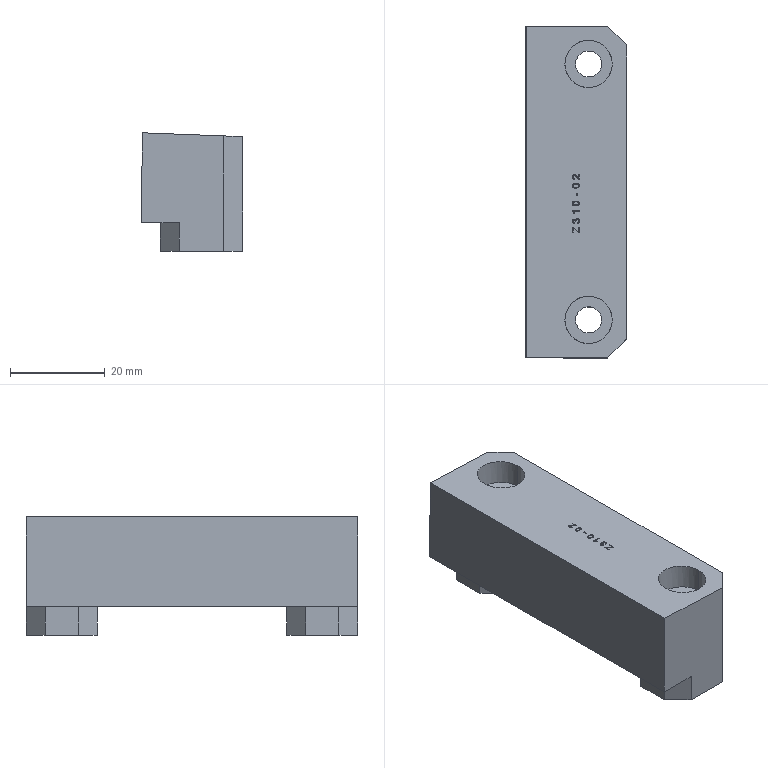Part | Creo | 1 solid | 156 faces | box 21.309 x 70 x 24.978 mm | volume 28277 mm3 | other 96 | plane 51 | cylinder 9 | commonest cylinder face diameters 5.5 x4 10 x4 20.538 x1